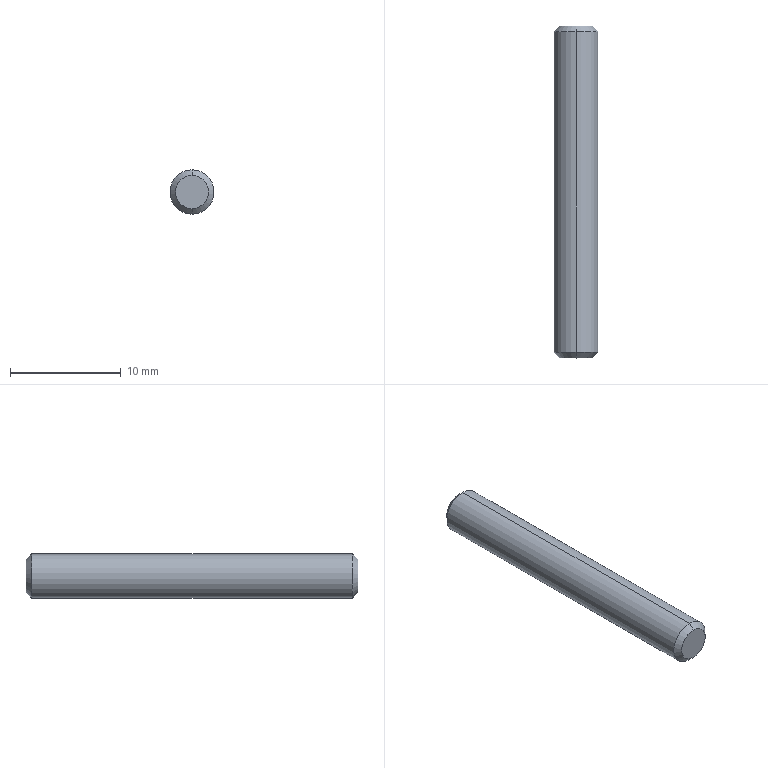Part | SolidWorks | features Chamfer 1, Extrusion 1 | 1 solid | 8 faces | box 4 x 30 x 4 mm | volume 374.111 mm3 | cone 4 | cylinder 2 | plane 2 | commonest cylinder face diameters 4 x2
STEP:
#1=CARTESIAN_POINT('',(0.,0.,1.5));
#2=VERTEX_POINT('',#1);
#3=CARTESIAN_POINT('',(0.,0.,-1.5));
#4=VERTEX_POINT('',#3);
#5=CARTESIAN_POINT('',(0.,0.,0.));
#6=DIRECTION('',(0.,1.,0.));
#7=DIRECTION('',(0.,0.,1.));
#8=AXIS2_PLACEMENT_3D('',#5,#6,#7);
#9=CIRCLE('',#8,1.5);
#10=EDGE_CURVE('',#2,#4,#9,.T.);
#11=ORIENTED_EDGE('',*,*,#10,.F.);
#12=CARTESIAN_POINT('',(0.,-0.5,2.));
#13=VERTEX_POINT('',#12);
#14=CARTESIAN_POINT('',(0.,0.,1.5));
#15=DIRECTION('',(0.,-0.7071,0.7071));
#16=VECTOR('',#15,1000.);
#17=LINE('',#14,#16);
#18=EDGE_CURVE('',#2,#13,#17,.T.);
#19=ORIENTED_EDGE('',*,*,#18,.T.);
#20=CARTESIAN_POINT('',(0.,-0.5,-2.));
#21=VERTEX_POINT('',#20);
#22=CARTESIAN_POINT('',(0.,-0.5,0.));
#23=DIRECTION('',(0.,-1.,0.));
#24=DIRECTION('',(0.,0.,1.));
#25=AXIS2_PLACEMENT_3D('',#22,#23,#24);
#26=CIRCLE('',#25,2.);
#27=EDGE_CURVE('',#21,#13,#26,.T.);
#28=ORIENTED_EDGE('',*,*,#27,.F.);
#29=CARTESIAN_POINT('',(0.,0.,-1.5));
#30=DIRECTION('',(0.,-0.7071,-0.7071));
#31=VECTOR('',#30,1000.);
#32=LINE('',#29,#31);
#33=EDGE_CURVE('',#4,#21,#32,.T.);
#34=ORIENTED_EDGE('',*,*,#33,.F.);
#35=EDGE_LOOP('',(#11,#19,#28,#34));
#36=FACE_OUTER_BOUND('',#35,.T.);
#37=CARTESIAN_POINT('',(0.,0.,0.));
#38=DIRECTION('',(0.,-1.,0.));
#39=DIRECTION('',(0.,0.,-1.));
#40=AXIS2_PLACEMENT_3D('',#37,#38,#39);
#41=CONICAL_SURFACE('',#40,1.5,0.7854);
#42=ADVANCED_FACE('',(#36),#41,.T.);
#43=CARTESIAN_POINT('',(0.,-30.,-1.5));
#44=VERTEX_POINT('',#43);
#45=CARTESIAN_POINT('',(0.,-30.,1.5));
#46=VERTEX_POINT('',#45);
#47=CARTESIAN_POINT('',(0.,-30.,0.));
#48=DIRECTION('',(0.,-1.,0.));
#49=DIRECTION('',(0.,0.,1.));
#50=AXIS2_PLACEMENT_3D('',#47,#48,#49);
#51=CIRCLE('',#50,1.5);
#52=EDGE_CURVE('',#44,#46,#51,.T.);
#53=ORIENTED_EDGE('',*,*,#52,.F.);
#54=CARTESIAN_POINT('',(0.,-29.5,-2.));
#55=VERTEX_POINT('',#54);
#56=CARTESIAN_POINT('',(0.,-29.5,-2.));
#57=DIRECTION('',(0.,0.7071,-0.7071));
#58=VECTOR('',#57,1000.);
#59=LINE('',#56,#58);
#60=EDGE_CURVE('',#44,#55,#59,.T.);
#61=ORIENTED_EDGE('',*,*,#60,.T.);
#62=CARTESIAN_POINT('',(0.,-29.5,2.));
#63=VERTEX_POINT('',#62);
#64=CARTESIAN_POINT('',(0.,-29.5,0.));
#65=DIRECTION('',(0.,1.,0.));
#66=DIRECTION('',(0.,0.,1.));
#67=AXIS2_PLACEMENT_3D('',#64,#65,#66);
#68=CIRCLE('',#67,2.);
#69=EDGE_CURVE('',#63,#55,#68,.T.);
#70=ORIENTED_EDGE('',*,*,#69,.F.);
#71=CARTESIAN_POINT('',(0.,-29.5,2.));
#72=DIRECTION('',(0.,0.7071,0.7071));
#73=VECTOR('',#72,1000.);
#74=LINE('',#71,#73);
#75=EDGE_CURVE('',#46,#63,#74,.T.);
#76=ORIENTED_EDGE('',*,*,#75,.F.);
#77=EDGE_LOOP('',(#53,#61,#70,#76));
#78=FACE_OUTER_BOUND('',#77,.T.);
#79=CARTESIAN_POINT('',(0.,-29.5,0.));
#80=DIRECTION('',(0.,1.,0.));
#81=DIRECTION('',(0.,0.,1.));
#82=AXIS2_PLACEMENT_3D('',#79,#80,#81);
#83=CONICAL_SURFACE('',#82,2.,0.7854);
#84=ADVANCED_FACE('',(#78),#83,.T.);
#85=ORIENTED_EDGE('',*,*,#69,.T.);
#86=CARTESIAN_POINT('',(0.,-30.,-2.));
#87=DIRECTION('',(0.,1.,0.));
#88=VECTOR('',#87,1000.);
#89=LINE('',#86,#88);
#90=EDGE_CURVE('',#55,#21,#89,.T.);
#91=ORIENTED_EDGE('',*,*,#90,.T.);
#92=ORIENTED_EDGE('',*,*,#27,.T.);
#93=CARTESIAN_POINT('',(0.,-30.,2.));
#94=DIRECTION('',(0.,1.,0.));
#95=VECTOR('',#94,1000.);
#96=LINE('',#93,#95);
#97=EDGE_CURVE('',#63,#13,#96,.T.);
#98=ORIENTED_EDGE('',*,*,#97,.F.);
#99=EDGE_LOOP('',(#85,#91,#92,#98));
#100=FACE_OUTER_BOUND('',#99,.T.);
#101=CARTESIAN_POINT('',(0.,-30.,0.));
#102=DIRECTION('',(0.,1.,0.));
#103=DIRECTION('',(0.,0.,1.));
#104=AXIS2_PLACEMENT_3D('',#101,#102,#103);
#105=CYLINDRICAL_SURFACE('',#104,2.);
#106=ADVANCED_FACE('',(#100),#105,.T.);
#107=ORIENTED_EDGE('',*,*,#90,.F.);
#108=CARTESIAN_POINT('',(0.,-29.5,0.));
#109=DIRECTION('',(0.,1.,0.));
#110=DIRECTION('',(0.,0.,1.));
#111=AXIS2_PLACEMENT_3D('',#108,#109,#110);
#112=CIRCLE('',#111,2.);
#113=EDGE_CURVE('',#55,#63,#112,.T.);
#114=ORIENTED_EDGE('',*,*,#113,.T.);
#115=ORIENTED_EDGE('',*,*,#97,.T.);
#116=CARTESIAN_POINT('',(0.,-0.5,0.));
#117=DIRECTION('',(0.,-1.,0.));
#118=DIRECTION('',(0.,0.,1.));
#119=AXIS2_PLACEMENT_3D('',#116,#117,#118);
#120=CIRCLE('',#119,2.);
#121=EDGE_CURVE('',#13,#21,#120,.T.);
#122=ORIENTED_EDGE('',*,*,#121,.T.);
#123=EDGE_LOOP('',(#107,#114,#115,#122));
#124=FACE_OUTER_BOUND('',#123,.T.);
#125=CARTESIAN_POINT('',(0.,-30.,0.));
#126=DIRECTION('',(0.,1.,0.));
#127=DIRECTION('',(0.,0.,1.));
#128=AXIS2_PLACEMENT_3D('',#125,#126,#127);
#129=CYLINDRICAL_SURFACE('',#128,2.);
#130=ADVANCED_FACE('',(#124),#129,.T.);
#131=CARTESIAN_POINT('',(0.,-30.,0.));
#132=DIRECTION('',(0.,-1.,0.));
#133=DIRECTION('',(0.,0.,1.));
#134=AXIS2_PLACEMENT_3D('',#131,#132,#133);
#135=CIRCLE('',#134,1.5);
#136=EDGE_CURVE('',#46,#44,#135,.T.);
#137=ORIENTED_EDGE('',*,*,#136,.T.);
#138=ORIENTED_EDGE('',*,*,#52,.T.);
#139=EDGE_LOOP('',(#137,#138));
#140=FACE_OUTER_BOUND('',#139,.T.);
#141=CARTESIAN_POINT('',(0.,-30.,0.));
#142=DIRECTION('',(0.,1.,0.));
#143=DIRECTION('',(0.,0.,1.));
#144=AXIS2_PLACEMENT_3D('',#141,#142,#143);
#145=PLANE('',#144);
#146=ADVANCED_FACE('',(#140),#145,.F.);
#147=CARTESIAN_POINT('',(0.,0.,0.));
#148=DIRECTION('',(0.,1.,0.));
#149=DIRECTION('',(0.,0.,1.));
#150=AXIS2_PLACEMENT_3D('',#147,#148,#149);
#151=CIRCLE('',#150,1.5);
#152=EDGE_CURVE('',#4,#2,#151,.T.);
#153=ORIENTED_EDGE('',*,*,#152,.T.);
#154=ORIENTED_EDGE('',*,*,#10,.T.);
#155=EDGE_LOOP('',(#153,#154));
#156=FACE_OUTER_BOUND('',#155,.T.);
#157=CARTESIAN_POINT('',(0.,0.,0.));
#158=DIRECTION('',(0.,1.,0.));
#159=DIRECTION('',(0.,0.,1.));
#160=AXIS2_PLACEMENT_3D('',#157,#158,#159);
#161=PLANE('',#160);
#162=ADVANCED_FACE('',(#156),#161,.T.);
#163=ORIENTED_EDGE('',*,*,#60,.F.);
#164=ORIENTED_EDGE('',*,*,#136,.F.);
#165=ORIENTED_EDGE('',*,*,#75,.T.);
#166=ORIENTED_EDGE('',*,*,#113,.F.);
#167=EDGE_LOOP('',(#163,#164,#165,#166));
#168=FACE_OUTER_BOUND('',#167,.T.);
#169=CARTESIAN_POINT('',(0.,-29.5,0.));
#170=DIRECTION('',(0.,1.,0.));
#171=DIRECTION('',(0.,0.,1.));
#172=AXIS2_PLACEMENT_3D('',#169,#170,#171);
#173=CONICAL_SURFACE('',#172,2.,0.7854);
#174=ADVANCED_FACE('',(#168),#173,.T.);
#175=ORIENTED_EDGE('',*,*,#18,.F.);
#176=ORIENTED_EDGE('',*,*,#152,.F.);
#177=ORIENTED_EDGE('',*,*,#33,.T.);
#178=ORIENTED_EDGE('',*,*,#121,.F.);
#179=EDGE_LOOP('',(#175,#176,#177,#178));
#180=FACE_OUTER_BOUND('',#179,.T.);
#181=CARTESIAN_POINT('',(0.,0.,0.));
#182=DIRECTION('',(0.,-1.,0.));
#183=DIRECTION('',(0.,0.,-1.));
#184=AXIS2_PLACEMENT_3D('',#181,#182,#183);
#185=CONICAL_SURFACE('',#184,1.5,0.7854);
#186=ADVANCED_FACE('',(#180),#185,.T.);
#187=CLOSED_SHELL('',(#42,#84,#106,#130,#146,#162,#174,#186));
#188=MANIFOLD_SOLID_BREP('',#187);
#189=CARTESIAN_POINT('',(0.,0.,0.));
#190=DIRECTION('',(0.,0.,1.));
#191=DIRECTION('',(1.,0.,0.));
#192=AXIS2_PLACEMENT_3D('',#189,#190,#191);
#193=(LENGTH_UNIT()NAMED_UNIT(*)SI_UNIT(.MILLI.,.METRE.));
#194=UNCERTAINTY_MEASURE_WITH_UNIT(LENGTH_MEASURE(0.00001),#193,'','');
#195=(NAMED_UNIT(*)PLANE_ANGLE_UNIT()SI_UNIT($,.RADIAN.));
#196=(NAMED_UNIT(*)SI_UNIT($,.STERADIAN.)SOLID_ANGLE_UNIT());
#197=(GEOMETRIC_REPRESENTATION_CONTEXT(3)GLOBAL_UNCERTAINTY_ASSIGNED_CONTEXT((#194))GLOBAL_UNIT_ASSIGNED_CONTEXT((#193,#195,#196))REPRESENTATION_CONTEXT('',''));
#198=ADVANCED_BREP_SHAPE_REPRESENTATION('',(#188,#192),#197);